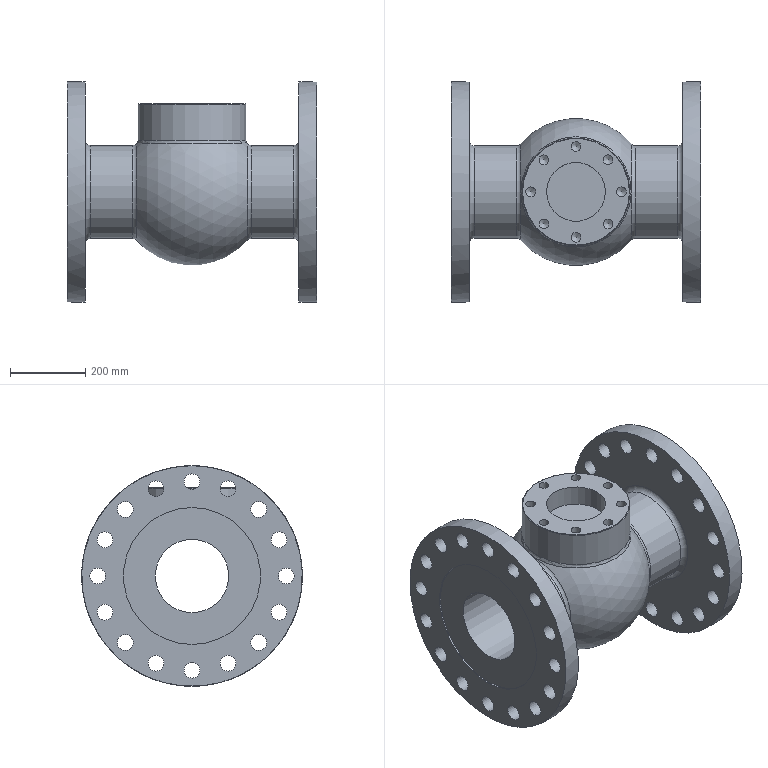Part | NX | features SKETCH 35, DATUM_CSYS 34, EXTRACT_DATUM_AXIS 32, EXTRACT_FACE 32, HOLE PACKAGE 32, SIMPLE HOLE 32, Instance Feature 15, ABSOLUTE_DATUM_AXIS 5, ABSOLUTE_DATUM_PLANE 5, Resize Face 3, EXTRUDE 2, AXIS_ANGLE_DATUM_PLANE 1, BREP 1, Pattern Feature 1 | 1 solid | 72 faces | box 660.4 x 585 x 585 mm | volume 47612449 mm3 | cylinder 49 | cone 9 | plane 8 | torus 5 | sphere 1 | commonest cylinder face diameters 42 x32 26 x8 247 x2 363 x2 585 x2 156 x1